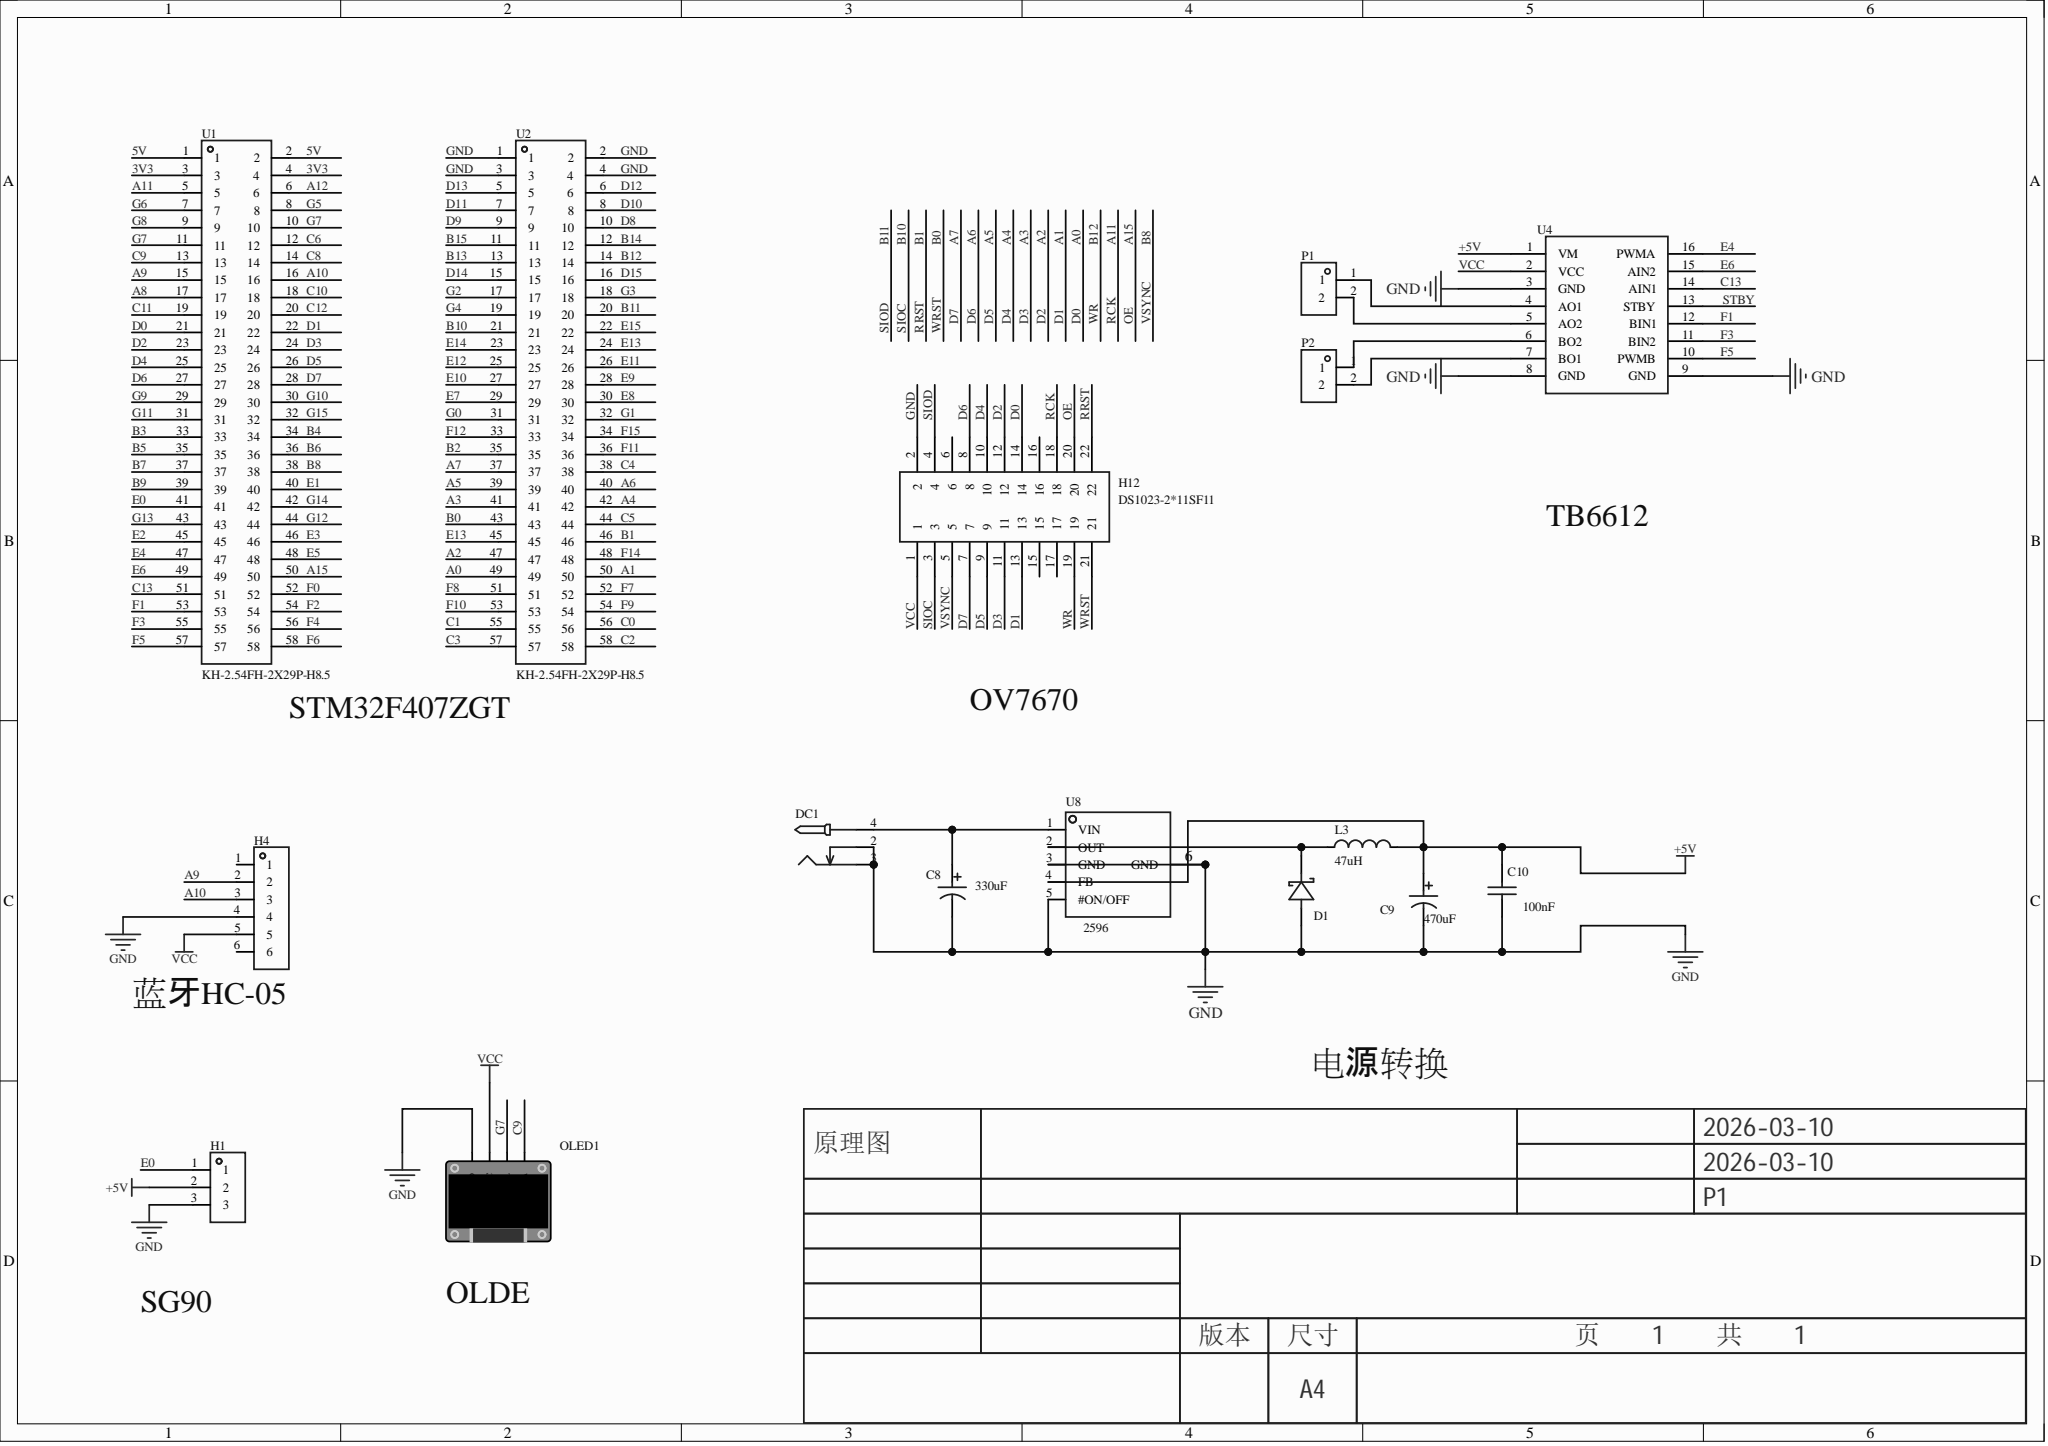Circuit board | Altium Designer | 16 parts | 39 nets
Bill of materials:
Comment,Description,Designator,Footprint,LibRef,Quantity
"","容值:220uF;精度:±20%;额定电压:35V;电容体直径:8mm;电容体长度:10.5mm;纹波电流:-;等效串联电阻:-;工作寿命:2000hrs@105;工作温度:-40~+105;","C8, C9","CAP-SMD_BD8.0-L8.3-W8.3-RD","CS1V221M-CRF10","2"
"","容值:100nF;精度:±10%;额定电压:50V;温度系数:X7R;","C10","C0805","CL21B104KBCNNNC","1"
"","","D1","SMA_L4.3-W2.6-LS5.2-RD","SS34_3","1"
"","","DC1","DC-2.0","DC-005_2.0","1"
"","","H1","HDR-TH_3P-P2.54-V-M","HDR-M_2.54_1x3P","1"
"","","H4","HDR-TH_6P-P2.54-V-F","HDR-F_2.54_1x6P","1"
"DS1023-2*11SF11","插孔结构:2x11P;间距:2.54mm;行距:2.54mm;安装方式:直插;排数:双排;总孔位数:22P;额定电流:3A;额定电压:600V;插孔方向:顶部;塑高:8.5mm;触头材质:-;触头镀层:金;工作温度:-40℃~+105℃;","H12","HDR-TH_22P-P2.54-V-F-R2-C11-S2.54","DS1023-2*11SF11","1"
"","","L3","IND-SMD_L7.0-W6.6","CMLO0630H330MTT","1"
"","","OLED1","0.96OLED_4P","0.96OLED模块_4P","1"
"KF301-2P接线端子","","P1, P2","CONN-TH_XY301V-A-5.0-2P","KF301-2P接线端子","2"
"KH-2.54FH-2X29P-H8.5","2.54FH H8.5 2x29Pin 180度 Y型 PC3.2 6T","U1, U2","HDR-TH_58P-P2.54-V-F-R2-C29-S2.54","KH-2.54FH-2X29P-H8.5","2"
"","","U4","tb6612","tb6612","1"
"LM2596S-5.0","功能类型:降压型;输出类型:固定;输入电压:40V;输出电压:5V;输出电流(最大值):3A;","U8","TO-263-5_L10.2-W8.9-P1.70-BR","LM2596S-5.0_C347421","1"
Netlist (Protel format):
[
C8
CAP-SMD_BD8.0-L8.3-W8.3-RD




]
[
C9
CAP-SMD_BD8.0-L8.3-W8.3-RD




]
[
C10
C0805




]
[
D1
SMA_L4.3-W2.6-LS5.2-RD




]
[
DC1
DC-2.0




]
[
H1
HDR-TH_3P-P2.54-V-M




]
[
H4
HDR-TH_6P-P2.54-V-F




]
[
H12
HDR-TH_22P-P2.54-V-F-R2-C11-S2.54
DS1023-2*11SF11



]
[
L3
IND-SMD_L7.0-W6.6




]
[
OLED1
0.96OLED_4P




]
[
P1
CONN-TH_XY301V-A-5.0-2P
KF301-2P接线端子



]
[
P2
CONN-TH_XY301V-A-5.0-2P
KF301-2P接线端子



]
[
U1
HDR-TH_58P-P2.54-V-F-R2-C29-S2.54
KH-2.54FH-2X29P-H8.5



]
[
U2
HDR-TH_58P-P2.54-V-F-R2-C29-S2.54
KH-2.54FH-2X29P-H8.5



]
[
U4
tb6612




]
[
U8
TO-263-5_L10.2-W8.9-P1.70-BR
LM2596S-5.0



]
(
VCC
H4-5
H12-1
OLED1-2
U4-2
)
(
NetP2_2
P2-2
U4-7
)
(
NetP2_1
P2-1
U4-6
)
(
NetP1_2
P1-2
U4-5
)
(
NetP1_1
P1-1
U4-4
)
(
NetD1_1
D1-1
L3-1
U8-2
)
(
NetC8_1
C8-1
DC1-4
U8-1
)
(
GND
C8-2
C9-2
C10-2
D1-2
DC1-2
DC1-3
H1-3
H4-4
H12-2
OLED1-1
U2-1
U2-2
U2-3
U2-4
U4-3
U4-8
U4-9
U8-3
U8-5
U8-6
)
(
G7
OLED1-3
U1-10
U1-11
)
(
F5
U1-57
U4-10
)
(
F3
U1-55
U4-11
)
(
F1
U1-53
U4-12
)
(
E13
U2-24
U2-45
)
(
E6
U1-49
U4-15
)
(
E4
U1-47
U4-16
)
(
E0
H1-1
U1-41
)
(
C13
U1-51
U4-14
)
(
C9
OLED1-4
U1-13
)
(
B12
H12-19
U2-14
)
(
B11
H12-4
U2-20
)
(
B10
H12-3
U2-21
)
(
B8
H12-5
U1-38
)
(
B1
H12-22
U2-46
)
(
B0
H12-21
U2-43
)
(
A15
H12-20
U1-50
)
(
A11
H12-18
U1-5
)
(
A10
H4-3
U1-16
)
(
A9
H4-2
U1-15
)
(
A7
H12-7
U1-28
U2-37
)
(
A6
H12-8
U1-27
U2-40
)
(
A5
H12-9
U1-26
U2-39
)
(
A4
H12-10
U1-25
U2-42
)
(
A3
H12-11
U1-24
U2-41
)
(
A2
H12-12
U1-23
U2-47
)
(
A1
H12-13
U1-22
U2-50
)
(
A0
H12-14
U1-21
U2-49
)
(
+5V
C9-1
C10-1
H1-2
L3-2
U4-1
U8-4
)
(
5V
U1-1
U1-2
)
(
3V3
U1-3
U1-4
)